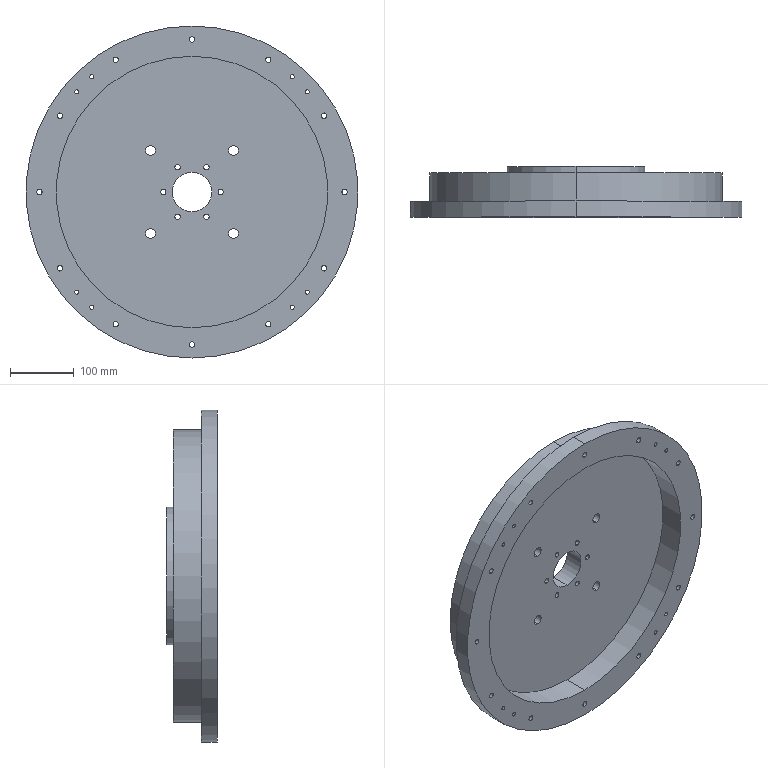Part | STEP file | 1 solid | 78 faces | box 520 x 79.32 x 520 mm | volume 7165293 mm3 | cylinder 72 | plane 6 | commonest cylinder face diameters 8.5 x36 6.5 x16 15.5 x8 62 x2 108 x2 215.9 x2